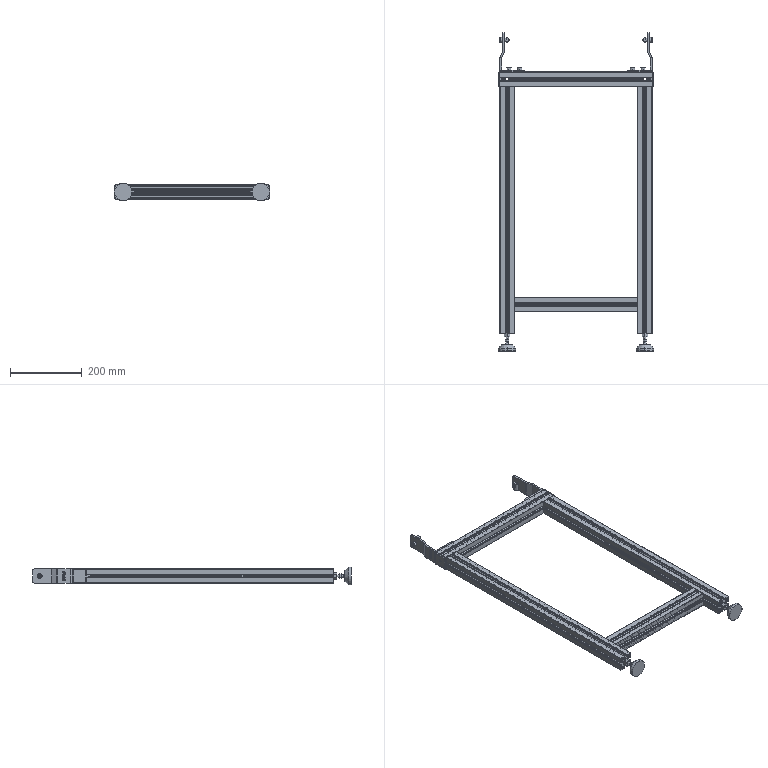Part | SolidWorks | features ReferencePattern 5, CoordSys 2, AEMSimFeature 1, MirrorCompFeat 1, RefPoint 1 | 30 solids | 2090 faces | box 435 x 890.5 x 50 mm | volume 1613187 mm3 | plane 1171 | cylinder 623 | spline 212 | cone 48 | torus 20 | sphere 16 | commonest cylinder face diameters 1 x184 0.6 x155 4 x52 4.9 x32 6.8 x28 8 x28